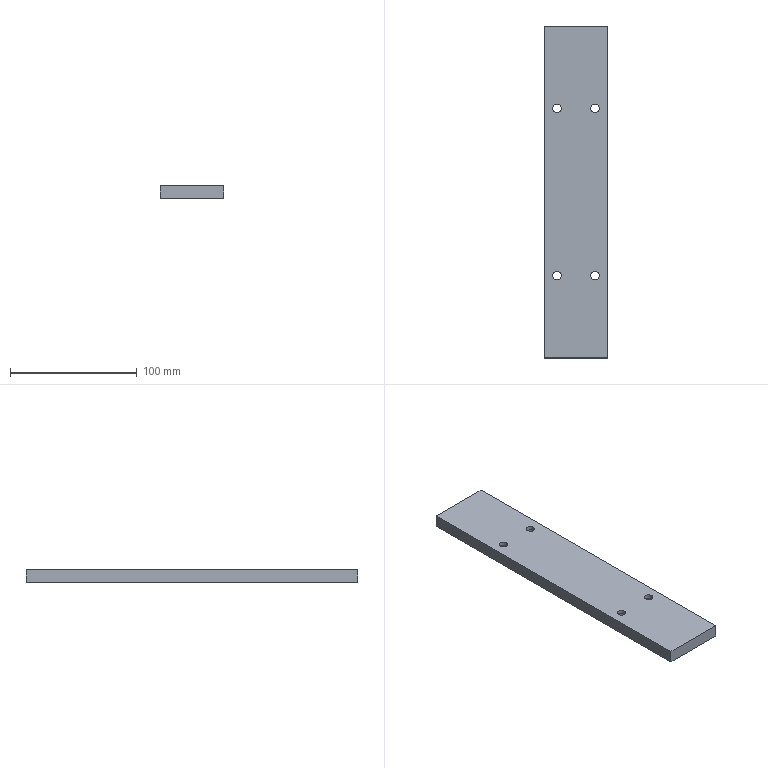Part | SolidWorks | features BaseBody 1 | 1 solid | 26 faces | box 50 x 262 x 10 mm | volume 127977 mm3 | cylinder 16 | plane 10 | commonest cylinder face diameters 6.6 x8 11 x8
STEP:
#1=CARTESIAN_POINT('',(-9.5,309.,-233.2));
#2=VERTEX_POINT('',#1);
#3=CARTESIAN_POINT('',(-20.5,309.,-233.2));
#4=VERTEX_POINT('',#3);
#5=CARTESIAN_POINT('',(-15.,309.,-233.2));
#6=DIRECTION('',(0.,0.,-1.));
#7=DIRECTION('',(-1.,0.,0.));
#8=AXIS2_PLACEMENT_3D('',#5,#6,#7);
#9=CIRCLE('',#8,5.5);
#10=EDGE_CURVE('',#2,#4,#9,.T.);
#11=ORIENTED_EDGE('',*,*,#10,.F.);
#12=CARTESIAN_POINT('',(-9.5,309.,-240.));
#13=VERTEX_POINT('',#12);
#14=CARTESIAN_POINT('',(-9.5,309.,-240.));
#15=DIRECTION('',(0.,0.,-1.));
#16=VECTOR('',#15,1000.);
#17=LINE('',#14,#16);
#18=EDGE_CURVE('',#2,#13,#17,.T.);
#19=ORIENTED_EDGE('',*,*,#18,.T.);
#20=CARTESIAN_POINT('',(-20.5,309.,-240.));
#21=VERTEX_POINT('',#20);
#22=CARTESIAN_POINT('',(-15.,309.,-240.));
#23=DIRECTION('',(0.,0.,-1.));
#24=DIRECTION('',(-1.,0.,0.));
#25=AXIS2_PLACEMENT_3D('',#22,#23,#24);
#26=CIRCLE('',#25,5.5);
#27=EDGE_CURVE('',#13,#21,#26,.T.);
#28=ORIENTED_EDGE('',*,*,#27,.T.);
#29=CARTESIAN_POINT('',(-20.5,309.,-240.));
#30=DIRECTION('',(0.,0.,-1.));
#31=VECTOR('',#30,1000.);
#32=LINE('',#29,#31);
#33=EDGE_CURVE('',#4,#21,#32,.T.);
#34=ORIENTED_EDGE('',*,*,#33,.F.);
#35=EDGE_LOOP('',(#11,#19,#28,#34));
#36=FACE_OUTER_BOUND('',#35,.T.);
#37=CARTESIAN_POINT('',(-15.,309.,-240.));
#38=DIRECTION('',(0.,0.,-1.));
#39=DIRECTION('',(-1.,0.,0.));
#40=AXIS2_PLACEMENT_3D('',#37,#38,#39);
#41=CYLINDRICAL_SURFACE('',#40,5.5);
#42=ADVANCED_FACE('',(#36),#41,.F.);
#43=CARTESIAN_POINT('',(-11.7,309.,-230.));
#44=VERTEX_POINT('',#43);
#45=CARTESIAN_POINT('',(-18.3,309.,-230.));
#46=VERTEX_POINT('',#45);
#47=CARTESIAN_POINT('',(-15.,309.,-230.));
#48=DIRECTION('',(0.,0.,-1.));
#49=DIRECTION('',(-1.,0.,0.));
#50=AXIS2_PLACEMENT_3D('',#47,#48,#49);
#51=CIRCLE('',#50,3.3);
#52=EDGE_CURVE('',#44,#46,#51,.T.);
#53=ORIENTED_EDGE('',*,*,#52,.F.);
#54=CARTESIAN_POINT('',(-11.7,309.,-233.2));
#55=VERTEX_POINT('',#54);
#56=CARTESIAN_POINT('',(-11.7,309.,-240.));
#57=DIRECTION('',(0.,0.,-1.));
#58=VECTOR('',#57,1000.);
#59=LINE('',#56,#58);
#60=EDGE_CURVE('',#44,#55,#59,.T.);
#61=ORIENTED_EDGE('',*,*,#60,.T.);
#62=CARTESIAN_POINT('',(-18.3,309.,-233.2));
#63=VERTEX_POINT('',#62);
#64=CARTESIAN_POINT('',(-15.,309.,-233.2));
#65=DIRECTION('',(0.,0.,-1.));
#66=DIRECTION('',(-1.,0.,0.));
#67=AXIS2_PLACEMENT_3D('',#64,#65,#66);
#68=CIRCLE('',#67,3.3);
#69=EDGE_CURVE('',#55,#63,#68,.T.);
#70=ORIENTED_EDGE('',*,*,#69,.T.);
#71=CARTESIAN_POINT('',(-18.3,309.,-240.));
#72=DIRECTION('',(0.,0.,-1.));
#73=VECTOR('',#72,1000.);
#74=LINE('',#71,#73);
#75=EDGE_CURVE('',#46,#63,#74,.T.);
#76=ORIENTED_EDGE('',*,*,#75,.F.);
#77=EDGE_LOOP('',(#53,#61,#70,#76));
#78=FACE_OUTER_BOUND('',#77,.T.);
#79=CARTESIAN_POINT('',(-15.,309.,-240.));
#80=DIRECTION('',(0.,0.,-1.));
#81=DIRECTION('',(-1.,0.,0.));
#82=AXIS2_PLACEMENT_3D('',#79,#80,#81);
#83=CYLINDRICAL_SURFACE('',#82,3.3);
#84=ADVANCED_FACE('',(#78),#83,.F.);
#85=CARTESIAN_POINT('',(20.5,309.,-233.2));
#86=VERTEX_POINT('',#85);
#87=CARTESIAN_POINT('',(9.5,309.,-233.2));
#88=VERTEX_POINT('',#87);
#89=CARTESIAN_POINT('',(15.,309.,-233.2));
#90=DIRECTION('',(0.,0.,-1.));
#91=DIRECTION('',(-1.,0.,0.));
#92=AXIS2_PLACEMENT_3D('',#89,#90,#91);
#93=CIRCLE('',#92,5.5);
#94=EDGE_CURVE('',#86,#88,#93,.T.);
#95=ORIENTED_EDGE('',*,*,#94,.F.);
#96=CARTESIAN_POINT('',(20.5,309.,-240.));
#97=VERTEX_POINT('',#96);
#98=CARTESIAN_POINT('',(20.5,309.,-240.));
#99=DIRECTION('',(0.,0.,-1.));
#100=VECTOR('',#99,1000.);
#101=LINE('',#98,#100);
#102=EDGE_CURVE('',#86,#97,#101,.T.);
#103=ORIENTED_EDGE('',*,*,#102,.T.);
#104=CARTESIAN_POINT('',(9.5,309.,-240.));
#105=VERTEX_POINT('',#104);
#106=CARTESIAN_POINT('',(15.,309.,-240.));
#107=DIRECTION('',(0.,0.,-1.));
#108=DIRECTION('',(-1.,0.,0.));
#109=AXIS2_PLACEMENT_3D('',#106,#107,#108);
#110=CIRCLE('',#109,5.5);
#111=EDGE_CURVE('',#97,#105,#110,.T.);
#112=ORIENTED_EDGE('',*,*,#111,.T.);
#113=CARTESIAN_POINT('',(9.5,309.,-240.));
#114=DIRECTION('',(0.,0.,-1.));
#115=VECTOR('',#114,1000.);
#116=LINE('',#113,#115);
#117=EDGE_CURVE('',#88,#105,#116,.T.);
#118=ORIENTED_EDGE('',*,*,#117,.F.);
#119=EDGE_LOOP('',(#95,#103,#112,#118));
#120=FACE_OUTER_BOUND('',#119,.T.);
#121=CARTESIAN_POINT('',(15.,309.,-240.));
#122=DIRECTION('',(0.,0.,-1.));
#123=DIRECTION('',(-1.,0.,0.));
#124=AXIS2_PLACEMENT_3D('',#121,#122,#123);
#125=CYLINDRICAL_SURFACE('',#124,5.5);
#126=ADVANCED_FACE('',(#120),#125,.F.);
#127=CARTESIAN_POINT('',(18.3,309.,-230.));
#128=VERTEX_POINT('',#127);
#129=CARTESIAN_POINT('',(11.7,309.,-230.));
#130=VERTEX_POINT('',#129);
#131=CARTESIAN_POINT('',(15.,309.,-230.));
#132=DIRECTION('',(0.,0.,-1.));
#133=DIRECTION('',(-1.,0.,0.));
#134=AXIS2_PLACEMENT_3D('',#131,#132,#133);
#135=CIRCLE('',#134,3.3);
#136=EDGE_CURVE('',#128,#130,#135,.T.);
#137=ORIENTED_EDGE('',*,*,#136,.F.);
#138=CARTESIAN_POINT('',(18.3,309.,-233.2));
#139=VERTEX_POINT('',#138);
#140=CARTESIAN_POINT('',(18.3,309.,-240.));
#141=DIRECTION('',(0.,0.,-1.));
#142=VECTOR('',#141,1000.);
#143=LINE('',#140,#142);
#144=EDGE_CURVE('',#128,#139,#143,.T.);
#145=ORIENTED_EDGE('',*,*,#144,.T.);
#146=CARTESIAN_POINT('',(11.7,309.,-233.2));
#147=VERTEX_POINT('',#146);
#148=CARTESIAN_POINT('',(15.,309.,-233.2));
#149=DIRECTION('',(0.,0.,-1.));
#150=DIRECTION('',(-1.,0.,0.));
#151=AXIS2_PLACEMENT_3D('',#148,#149,#150);
#152=CIRCLE('',#151,3.3);
#153=EDGE_CURVE('',#139,#147,#152,.T.);
#154=ORIENTED_EDGE('',*,*,#153,.T.);
#155=CARTESIAN_POINT('',(11.7,309.,-240.));
#156=DIRECTION('',(0.,0.,-1.));
#157=VECTOR('',#156,1000.);
#158=LINE('',#155,#157);
#159=EDGE_CURVE('',#130,#147,#158,.T.);
#160=ORIENTED_EDGE('',*,*,#159,.F.);
#161=EDGE_LOOP('',(#137,#145,#154,#160));
#162=FACE_OUTER_BOUND('',#161,.T.);
#163=CARTESIAN_POINT('',(15.,309.,-240.));
#164=DIRECTION('',(0.,0.,-1.));
#165=DIRECTION('',(-1.,0.,0.));
#166=AXIS2_PLACEMENT_3D('',#163,#164,#165);
#167=CYLINDRICAL_SURFACE('',#166,3.3);
#168=ADVANCED_FACE('',(#162),#167,.F.);
#169=CARTESIAN_POINT('',(18.3,441.,-230.));
#170=VERTEX_POINT('',#169);
#171=CARTESIAN_POINT('',(11.7,441.,-230.));
#172=VERTEX_POINT('',#171);
#173=CARTESIAN_POINT('',(15.,441.,-230.));
#174=DIRECTION('',(0.,0.,-1.));
#175=DIRECTION('',(-1.,0.,0.));
#176=AXIS2_PLACEMENT_3D('',#173,#174,#175);
#177=CIRCLE('',#176,3.3);
#178=EDGE_CURVE('',#170,#172,#177,.T.);
#179=ORIENTED_EDGE('',*,*,#178,.F.);
#180=CARTESIAN_POINT('',(18.3,441.,-233.2));
#181=VERTEX_POINT('',#180);
#182=CARTESIAN_POINT('',(18.3,441.,-240.));
#183=DIRECTION('',(0.,0.,-1.));
#184=VECTOR('',#183,1000.);
#185=LINE('',#182,#184);
#186=EDGE_CURVE('',#170,#181,#185,.T.);
#187=ORIENTED_EDGE('',*,*,#186,.T.);
#188=CARTESIAN_POINT('',(11.7,441.,-233.2));
#189=VERTEX_POINT('',#188);
#190=CARTESIAN_POINT('',(15.,441.,-233.2));
#191=DIRECTION('',(0.,0.,-1.));
#192=DIRECTION('',(-1.,0.,0.));
#193=AXIS2_PLACEMENT_3D('',#190,#191,#192);
#194=CIRCLE('',#193,3.3);
#195=EDGE_CURVE('',#181,#189,#194,.T.);
#196=ORIENTED_EDGE('',*,*,#195,.T.);
#197=CARTESIAN_POINT('',(11.7,441.,-240.));
#198=DIRECTION('',(0.,0.,-1.));
#199=VECTOR('',#198,1000.);
#200=LINE('',#197,#199);
#201=EDGE_CURVE('',#172,#189,#200,.T.);
#202=ORIENTED_EDGE('',*,*,#201,.F.);
#203=EDGE_LOOP('',(#179,#187,#196,#202));
#204=FACE_OUTER_BOUND('',#203,.T.);
#205=CARTESIAN_POINT('',(15.,441.,-240.));
#206=DIRECTION('',(0.,0.,-1.));
#207=DIRECTION('',(-1.,0.,0.));
#208=AXIS2_PLACEMENT_3D('',#205,#206,#207);
#209=CYLINDRICAL_SURFACE('',#208,3.3);
#210=ADVANCED_FACE('',(#204),#209,.F.);
#211=CARTESIAN_POINT('',(20.5,441.,-233.2));
#212=VERTEX_POINT('',#211);
#213=CARTESIAN_POINT('',(9.5,441.,-233.2));
#214=VERTEX_POINT('',#213);
#215=CARTESIAN_POINT('',(15.,441.,-233.2));
#216=DIRECTION('',(0.,0.,-1.));
#217=DIRECTION('',(-1.,0.,0.));
#218=AXIS2_PLACEMENT_3D('',#215,#216,#217);
#219=CIRCLE('',#218,5.5);
#220=EDGE_CURVE('',#212,#214,#219,.T.);
#221=ORIENTED_EDGE('',*,*,#220,.F.);
#222=CARTESIAN_POINT('',(20.5,441.,-240.));
#223=VERTEX_POINT('',#222);
#224=CARTESIAN_POINT('',(20.5,441.,-240.));
#225=DIRECTION('',(0.,0.,-1.));
#226=VECTOR('',#225,1000.);
#227=LINE('',#224,#226);
#228=EDGE_CURVE('',#212,#223,#227,.T.);
#229=ORIENTED_EDGE('',*,*,#228,.T.);
#230=CARTESIAN_POINT('',(9.5,441.,-240.));
#231=VERTEX_POINT('',#230);
#232=CARTESIAN_POINT('',(15.,441.,-240.));
#233=DIRECTION('',(0.,0.,-1.));
#234=DIRECTION('',(-1.,0.,0.));
#235=AXIS2_PLACEMENT_3D('',#232,#233,#234);
#236=CIRCLE('',#235,5.5);
#237=EDGE_CURVE('',#223,#231,#236,.T.);
#238=ORIENTED_EDGE('',*,*,#237,.T.);
#239=CARTESIAN_POINT('',(9.5,441.,-240.));
#240=DIRECTION('',(0.,0.,-1.));
#241=VECTOR('',#240,1000.);
#242=LINE('',#239,#241);
#243=EDGE_CURVE('',#214,#231,#242,.T.);
#244=ORIENTED_EDGE('',*,*,#243,.F.);
#245=EDGE_LOOP('',(#221,#229,#238,#244));
#246=FACE_OUTER_BOUND('',#245,.T.);
#247=CARTESIAN_POINT('',(15.,441.,-240.));
#248=DIRECTION('',(0.,0.,-1.));
#249=DIRECTION('',(-1.,0.,0.));
#250=AXIS2_PLACEMENT_3D('',#247,#248,#249);
#251=CYLINDRICAL_SURFACE('',#250,5.5);
#252=ADVANCED_FACE('',(#246),#251,.F.);
#253=CARTESIAN_POINT('',(-11.7,441.,-230.));
#254=VERTEX_POINT('',#253);
#255=CARTESIAN_POINT('',(-18.3,441.,-230.));
#256=VERTEX_POINT('',#255);
#257=CARTESIAN_POINT('',(-15.,441.,-230.));
#258=DIRECTION('',(0.,0.,-1.));
#259=DIRECTION('',(-1.,0.,0.));
#260=AXIS2_PLACEMENT_3D('',#257,#258,#259);
#261=CIRCLE('',#260,3.3);
#262=EDGE_CURVE('',#254,#256,#261,.T.);
#263=ORIENTED_EDGE('',*,*,#262,.F.);
#264=CARTESIAN_POINT('',(-11.7,441.,-233.2));
#265=VERTEX_POINT('',#264);
#266=CARTESIAN_POINT('',(-11.7,441.,-240.));
#267=DIRECTION('',(0.,0.,-1.));
#268=VECTOR('',#267,1000.);
#269=LINE('',#266,#268);
#270=EDGE_CURVE('',#254,#265,#269,.T.);
#271=ORIENTED_EDGE('',*,*,#270,.T.);
#272=CARTESIAN_POINT('',(-18.3,441.,-233.2));
#273=VERTEX_POINT('',#272);
#274=CARTESIAN_POINT('',(-15.,441.,-233.2));
#275=DIRECTION('',(0.,0.,-1.));
#276=DIRECTION('',(-1.,0.,0.));
#277=AXIS2_PLACEMENT_3D('',#274,#275,#276);
#278=CIRCLE('',#277,3.3);
#279=EDGE_CURVE('',#265,#273,#278,.T.);
#280=ORIENTED_EDGE('',*,*,#279,.T.);
#281=CARTESIAN_POINT('',(-18.3,441.,-240.));
#282=DIRECTION('',(0.,0.,-1.));
#283=VECTOR('',#282,1000.);
#284=LINE('',#281,#283);
#285=EDGE_CURVE('',#256,#273,#284,.T.);
#286=ORIENTED_EDGE('',*,*,#285,.F.);
#287=EDGE_LOOP('',(#263,#271,#280,#286));
#288=FACE_OUTER_BOUND('',#287,.T.);
#289=CARTESIAN_POINT('',(-15.,441.,-240.));
#290=DIRECTION('',(0.,0.,-1.));
#291=DIRECTION('',(-1.,0.,0.));
#292=AXIS2_PLACEMENT_3D('',#289,#290,#291);
#293=CYLINDRICAL_SURFACE('',#292,3.3);
#294=ADVANCED_FACE('',(#288),#293,.F.);
#295=CARTESIAN_POINT('',(-9.5,441.,-233.2));
#296=VERTEX_POINT('',#295);
#297=CARTESIAN_POINT('',(-20.5,441.,-233.2));
#298=VERTEX_POINT('',#297);
#299=CARTESIAN_POINT('',(-15.,441.,-233.2));
#300=DIRECTION('',(0.,0.,-1.));
#301=DIRECTION('',(-1.,0.,0.));
#302=AXIS2_PLACEMENT_3D('',#299,#300,#301);
#303=CIRCLE('',#302,5.5);
#304=EDGE_CURVE('',#296,#298,#303,.T.);
#305=ORIENTED_EDGE('',*,*,#304,.F.);
#306=CARTESIAN_POINT('',(-9.5,441.,-240.));
#307=VERTEX_POINT('',#306);
#308=CARTESIAN_POINT('',(-9.5,441.,-240.));
#309=DIRECTION('',(0.,0.,-1.));
#310=VECTOR('',#309,1000.);
#311=LINE('',#308,#310);
#312=EDGE_CURVE('',#296,#307,#311,.T.);
#313=ORIENTED_EDGE('',*,*,#312,.T.);
#314=CARTESIAN_POINT('',(-20.5,441.,-240.));
#315=VERTEX_POINT('',#314);
#316=CARTESIAN_POINT('',(-15.,441.,-240.));
#317=DIRECTION('',(0.,0.,-1.));
#318=DIRECTION('',(-1.,0.,0.));
#319=AXIS2_PLACEMENT_3D('',#316,#317,#318);
#320=CIRCLE('',#319,5.5);
#321=EDGE_CURVE('',#307,#315,#320,.T.);
#322=ORIENTED_EDGE('',*,*,#321,.T.);
#323=CARTESIAN_POINT('',(-20.5,441.,-240.));
#324=DIRECTION('',(0.,0.,-1.));
#325=VECTOR('',#324,1000.);
#326=LINE('',#323,#325);
#327=EDGE_CURVE('',#298,#315,#326,.T.);
#328=ORIENTED_EDGE('',*,*,#327,.F.);
#329=EDGE_LOOP('',(#305,#313,#322,#328));
#330=FACE_OUTER_BOUND('',#329,.T.);
#331=CARTESIAN_POINT('',(-15.,441.,-240.));
#332=DIRECTION('',(0.,0.,-1.));
#333=DIRECTION('',(-1.,0.,0.));
#334=AXIS2_PLACEMENT_3D('',#331,#332,#333);
#335=CYLINDRICAL_SURFACE('',#334,5.5);
#336=ADVANCED_FACE('',(#330),#335,.F.);
#337=CARTESIAN_POINT('',(-25.,244.,-240.));
#338=VERTEX_POINT('',#337);
#339=CARTESIAN_POINT('',(25.,244.,-240.));
#340=VERTEX_POINT('',#339);
#341=CARTESIAN_POINT('',(25.,244.,-240.));
#342=DIRECTION('',(1.,0.,0.));
#343=VECTOR('',#342,1000.);
#344=LINE('',#341,#343);
#345=EDGE_CURVE('',#338,#340,#344,.T.);
#346=ORIENTED_EDGE('',*,*,#345,.T.);
#347=CARTESIAN_POINT('',(25.,244.,-230.));
#348=VERTEX_POINT('',#347);
#349=CARTESIAN_POINT('',(25.,244.,-230.));
#350=DIRECTION('',(0.,0.,1.));
#351=VECTOR('',#350,1000.);
#352=LINE('',#349,#351);
#353=EDGE_CURVE('',#340,#348,#352,.T.);
#354=ORIENTED_EDGE('',*,*,#353,.T.);
#355=CARTESIAN_POINT('',(-25.,244.,-230.));
#356=VERTEX_POINT('',#355);
#357=CARTESIAN_POINT('',(25.,244.,-230.));
#358=DIRECTION('',(1.,0.,0.));
#359=VECTOR('',#358,1000.);
#360=LINE('',#357,#359);
#361=EDGE_CURVE('',#356,#348,#360,.T.);
#362=ORIENTED_EDGE('',*,*,#361,.F.);
#363=CARTESIAN_POINT('',(-25.,244.,-230.));
#364=DIRECTION('',(0.,0.,1.));
#365=VECTOR('',#364,1000.);
#366=LINE('',#363,#365);
#367=EDGE_CURVE('',#338,#356,#366,.T.);
#368=ORIENTED_EDGE('',*,*,#367,.F.);
#369=EDGE_LOOP('',(#346,#354,#362,#368));
#370=FACE_OUTER_BOUND('',#369,.T.);
#371=CARTESIAN_POINT('',(11453.619,244.,-234.));
#372=DIRECTION('',(0.,1.,0.));
#373=DIRECTION('',(1.,0.,0.));
#374=AXIS2_PLACEMENT_3D('',#371,#372,#373);
#375=PLANE('',#374);
#376=ADVANCED_FACE('',(#370),#375,.F.);
#377=CARTESIAN_POINT('',(25.,506.,-240.));
#378=VERTEX_POINT('',#377);
#379=CARTESIAN_POINT('',(-25.,506.,-240.));
#380=VERTEX_POINT('',#379);
#381=CARTESIAN_POINT('',(25.,506.,-240.));
#382=DIRECTION('',(-1.,0.,0.));
#383=VECTOR('',#382,1000.);
#384=LINE('',#381,#383);
#385=EDGE_CURVE('',#378,#380,#384,.T.);
#386=ORIENTED_EDGE('',*,*,#385,.T.);
#387=CARTESIAN_POINT('',(-25.,506.,-230.));
#388=VERTEX_POINT('',#387);
#389=CARTESIAN_POINT('',(-25.,506.,-230.));
#390=DIRECTION('',(0.,0.,1.));
#391=VECTOR('',#390,1000.);
#392=LINE('',#389,#391);
#393=EDGE_CURVE('',#380,#388,#392,.T.);
#394=ORIENTED_EDGE('',*,*,#393,.T.);
#395=CARTESIAN_POINT('',(25.,506.,-230.));
#396=VERTEX_POINT('',#395);
#397=CARTESIAN_POINT('',(25.,506.,-230.));
#398=DIRECTION('',(-1.,0.,0.));
#399=VECTOR('',#398,1000.);
#400=LINE('',#397,#399);
#401=EDGE_CURVE('',#396,#388,#400,.T.);
#402=ORIENTED_EDGE('',*,*,#401,.F.);
#403=CARTESIAN_POINT('',(25.,506.,-230.));
#404=DIRECTION('',(0.,0.,1.));
#405=VECTOR('',#404,1000.);
#406=LINE('',#403,#405);
#407=EDGE_CURVE('',#378,#396,#406,.T.);
#408=ORIENTED_EDGE('',*,*,#407,.F.);
#409=EDGE_LOOP('',(#386,#394,#402,#408));
#410=FACE_OUTER_BOUND('',#409,.T.);
#411=CARTESIAN_POINT('',(-9973.619,506.,-234.));
#412=DIRECTION('',(0.,-1.,0.));
#413=DIRECTION('',(0.,0.,-1.));
#414=AXIS2_PLACEMENT_3D('',#411,#412,#413);
#415=PLANE('',#414);
#416=ADVANCED_FACE('',(#410),#415,.F.);
#417=CARTESIAN_POINT('',(-15.,309.,-233.2));
#418=DIRECTION('',(0.,0.,-1.));
#419=DIRECTION('',(-1.,0.,0.));
#420=AXIS2_PLACEMENT_3D('',#417,#418,#419);
#421=CIRCLE('',#420,3.3);
#422=EDGE_CURVE('',#63,#55,#421,.T.);
#423=ORIENTED_EDGE('',*,*,#422,.F.);
#424=ORIENTED_EDGE('',*,*,#69,.F.);
#425=EDGE_LOOP('',(#423,#424));
#426=FACE_BOUND('',#425,.T.);
#427=CARTESIAN_POINT('',(-15.,309.,-233.2));
#428=DIRECTION('',(0.,0.,-1.));
#429=DIRECTION('',(-1.,0.,0.));
#430=AXIS2_PLACEMENT_3D('',#427,#428,#429);
#431=CIRCLE('',#430,5.5);
#432=EDGE_CURVE('',#4,#2,#431,.T.);
#433=ORIENTED_EDGE('',*,*,#432,.T.);
#434=ORIENTED_EDGE('',*,*,#10,.T.);
#435=EDGE_LOOP('',(#433,#434));
#436=FACE_OUTER_BOUND('',#435,.T.);
#437=CARTESIAN_POINT('',(-11.7,309.,-233.2));
#438=DIRECTION('',(0.,0.,1.));
#439=DIRECTION('',(1.,0.,0.));
#440=AXIS2_PLACEMENT_3D('',#437,#438,#439);
#441=PLANE('',#440);
#442=ADVANCED_FACE('',(#426,#436),#441,.F.);
#443=CARTESIAN_POINT('',(15.,309.,-233.2));
#444=DIRECTION('',(0.,0.,-1.));
#445=DIRECTION('',(-1.,0.,0.));
#446=AXIS2_PLACEMENT_3D('',#443,#444,#445);
#447=CIRCLE('',#446,3.3);
#448=EDGE_CURVE('',#147,#139,#447,.T.);
#449=ORIENTED_EDGE('',*,*,#448,.F.);
#450=ORIENTED_EDGE('',*,*,#153,.F.);
#451=EDGE_LOOP('',(#449,#450));
#452=FACE_BOUND('',#451,.T.);
#453=CARTESIAN_POINT('',(15.,309.,-233.2));
#454=DIRECTION('',(0.,0.,-1.));
#455=DIRECTION('',(-1.,0.,0.));
#456=AXIS2_PLACEMENT_3D('',#453,#454,#455);
#457=CIRCLE('',#456,5.5);
#458=EDGE_CURVE('',#88,#86,#457,.T.);
#459=ORIENTED_EDGE('',*,*,#458,.T.);
#460=ORIENTED_EDGE('',*,*,#94,.T.);
#461=EDGE_LOOP('',(#459,#460));
#462=FACE_OUTER_BOUND('',#461,.T.);
#463=CARTESIAN_POINT('',(18.3,309.,-233.2));
#464=DIRECTION('',(0.,0.,1.));
#465=DIRECTION('',(1.,0.,0.));
#466=AXIS2_PLACEMENT_3D('',#463,#464,#465);
#467=PLANE('',#466);
#468=ADVANCED_FACE('',(#452,#462),#467,.F.);
#469=CARTESIAN_POINT('',(-15.,441.,-240.));
#470=DIRECTION('',(0.,0.,-1.));
#471=DIRECTION('',(-1.,0.,0.));
#472=AXIS2_PLACEMENT_3D('',#469,#470,#471);
#473=CIRCLE('',#472,5.5);
#474=EDGE_CURVE('',#315,#307,#473,.T.);
#475=ORIENTED_EDGE('',*,*,#474,.F.);
#476=ORIENTED_EDGE('',*,*,#321,.F.);
#477=EDGE_LOOP('',(#475,#476));
#478=FACE_BOUND('',#477,.T.);
#479=CARTESIAN_POINT('',(15.,441.,-240.));
#480=DIRECTION('',(0.,0.,-1.));
#481=DIRECTION('',(-1.,0.,0.));
#482=AXIS2_PLACEMENT_3D('',#479,#480,#481);
#483=CIRCLE('',#482,5.5);
#484=EDGE_CURVE('',#231,#223,#483,.T.);
#485=ORIENTED_EDGE('',*,*,#484,.F.);
#486=ORIENTED_EDGE('',*,*,#237,.F.);
#487=EDGE_LOOP('',(#485,#486));
#488=FACE_BOUND('',#487,.T.);
#489=CARTESIAN_POINT('',(15.,309.,-240.));
#490=DIRECTION('',(0.,0.,-1.));
#491=DIRECTION('',(-1.,0.,0.));
#492=AXIS2_PLACEMENT_3D('',#489,#490,#491);
#493=CIRCLE('',#492,5.5);
#494=EDGE_CURVE('',#105,#97,#493,.T.);
#495=ORIENTED_EDGE('',*,*,#494,.F.);
#496=ORIENTED_EDGE('',*,*,#111,.F.);
#497=EDGE_LOOP('',(#495,#496));
#498=FACE_BOUND('',#497,.T.);
#499=CARTESIAN_POINT('',(-15.,309.,-240.));
#500=DIRECTION('',(0.,0.,-1.));
#501=DIRECTION('',(-1.,0.,0.));
#502=AXIS2_PLACEMENT_3D('',#499,#500,#501);
#503=CIRCLE('',#502,5.5);
#504=EDGE_CURVE('',#21,#13,#503,.T.);
#505=ORIENTED_EDGE('',*,*,#504,.F.);
#506=ORIENTED_EDGE('',*,*,#27,.F.);
#507=EDGE_LOOP('',(#505,#506));
#508=FACE_BOUND('',#507,.T.);
#509=CARTESIAN_POINT('',(25.,496.,-240.));
#510=DIRECTION('',(0.,-1.,0.));
#511=VECTOR('',#510,1000.);
#512=LINE('',#509,#511);
#513=EDGE_CURVE('',#378,#340,#512,.T.);
#514=ORIENTED_EDGE('',*,*,#513,.T.);
#515=ORIENTED_EDGE('',*,*,#345,.F.);
#516=CARTESIAN_POINT('',(-25.,496.,-240.));
#517=DIRECTION('',(0.,1.,0.));
#518=VECTOR('',#517,1000.);
#519=LINE('',#516,#518);
#520=EDGE_CURVE('',#338,#380,#519,.T.);
#521=ORIENTED_EDGE('',*,*,#520,.T.);
#522=ORIENTED_EDGE('',*,*,#385,.F.);
#523=EDGE_LOOP('',(#514,#515,#521,#522));
#524=FACE_OUTER_BOUND('',#523,.T.);
#525=CARTESIAN_POINT('',(-1480.,0.,-240.));
#526=DIRECTION('',(0.,0.,-1.));
#527=DIRECTION('',(0.,-1.,0.));
#528=AXIS2_PLACEMENT_3D('',#525,#526,#527);
#529=PLANE('',#528);
#530=ADVANCED_FACE('',(#478,#488,#498,#508,#524),#529,.T.);
#531=CARTESIAN_POINT('',(-15.,441.,-230.));
#532=DIRECTION('',(0.,0.,-1.));
#533=DIRECTION('',(-1.,0.,0.));
#534=AXIS2_PLACEMENT_3D('',#531,#532,#533);
#535=CIRCLE('',#534,3.3);
#536=EDGE_CURVE('',#256,#254,#535,.T.);
#537=ORIENTED_EDGE('',*,*,#536,.T.);
#538=ORIENTED_EDGE('',*,*,#262,.T.);
#539=EDGE_LOOP('',(#537,#538));
#540=FACE_BOUND('',#539,.T.);
#541=CARTESIAN_POINT('',(15.,441.,-230.));
#542=DIRECTION('',(0.,0.,-1.));
#543=DIRECTION('',(-1.,0.,0.));
#544=AXIS2_PLACEMENT_3D('',#541,#542,#543);
#545=CIRCLE('',#544,3.3);
#546=EDGE_CURVE('',#172,#170,#545,.T.);
#547=ORIENTED_EDGE('',*,*,#546,.T.);
#548=ORIENTED_EDGE('',*,*,#178,.T.);
#549=EDGE_LOOP('',(#547,#548));
#550=FACE_BOUND('',#549,.T.);
#551=CARTESIAN_POINT('',(15.,309.,-230.));
#552=DIRECTION('',(0.,0.,-1.));
#553=DIRECTION('',(-1.,0.,0.));
#554=AXIS2_PLACEMENT_3D('',#551,#552,#553);
#555=CIRCLE('',#554,3.3);
#556=EDGE_CURVE('',#130,#128,#555,.T.);
#557=ORIENTED_EDGE('',*,*,#556,.T.);
#558=ORIENTED_EDGE('',*,*,#136,.T.);
#559=EDGE_LOOP('',(#557,#558));
#560=FACE_BOUND('',#559,.T.);
#561=CARTESIAN_POINT('',(-15.,309.,-230.));
#562=DIRECTION('',(0.,0.,-1.));
#563=DIRECTION('',(-1.,0.,0.));
#564=AXIS2_PLACEMENT_3D('',#561,#562,#563);
#565=CIRCLE('',#564,3.3);
#566=EDGE_CURVE('',#46,#44,#565,.T.);
#567=ORIENTED_EDGE('',*,*,#566,.T.);
#568=ORIENTED_EDGE('',*,*,#52,.T.);
#569=EDGE_LOOP('',(#567,#568));
#570=FACE_BOUND('',#569,.T.);
#571=CARTESIAN_POINT('',(25.,496.,-230.));
#572=DIRECTION('',(0.,-1.,0.));
#573=VECTOR('',#572,1000.);
#574=LINE('',#571,#573);
#575=EDGE_CURVE('',#396,#348,#574,.T.);
#576=ORIENTED_EDGE('',*,*,#575,.F.);
#577=ORIENTED_EDGE('',*,*,#401,.T.);
#578=CARTESIAN_POINT('',(-25.,496.,-230.));
#579=DIRECTION('',(0.,1.,0.));
#580=VECTOR('',#579,1000.);
#581=LINE('',#578,#580);
#582=EDGE_CURVE('',#356,#388,#581,.T.);
#583=ORIENTED_EDGE('',*,*,#582,.F.);
#584=ORIENTED_EDGE('',*,*,#361,.T.);
#585=EDGE_LOOP('',(#576,#577,#583,#584));
#586=FACE_OUTER_BOUND('',#585,.T.);
#587=CARTESIAN_POINT('',(-1480.,0.,-230.));
#588=DIRECTION('',(0.,0.,-1.));
#589=DIRECTION('',(0.,-1.,0.));
#590=AXIS2_PLACEMENT_3D('',#587,#588,#589);
#591=PLANE('',#590);
#592=ADVANCED_FACE('',(#540,#550,#560,#570,#586),#591,.F.);
#593=ORIENTED_EDGE('',*,*,#520,.F.);
#594=ORIENTED_EDGE('',*,*,#367,.T.);
#595=ORIENTED_EDGE('',*,*,#582,.T.);
#596=ORIENTED_EDGE('',*,*,#393,.F.);
#597=EDGE_LOOP('',(#593,#594,#595,#596));
#598=FACE_OUTER_BOUND('',#597,.T.);
#599=CARTESIAN_POINT('',(-25.,496.,-230.));
#600=DIRECTION('',(-1.,0.,0.));
#601=DIRECTION('',(0.,0.,1.));
#602=AXIS2_PLACEMENT_3D('',#599,#600,#601);
#603=PLANE('',#602);
#604=ADVANCED_FACE('',(#598),#603,.T.);
#605=ORIENTED_EDGE('',*,*,#513,.F.);
#606=ORIENTED_EDGE('',*,*,#407,.T.);
#607=ORIENTED_EDGE('',*,*,#575,.T.);
#608=ORIENTED_EDGE('',*,*,#353,.F.);
#609=EDGE_LOOP('',(#605,#606,#607,#608));
#610=FACE_OUTER_BOUND('',#609,.T.);
#611=CARTESIAN_POINT('',(25.,496.,-230.));
#612=DIRECTION('',(1.,0.,0.));
#613=DIRECTION('',(0.,1.,0.));
#614=AXIS2_PLACEMENT_3D('',#611,#612,#613);
#615=PLANE('',#614);
#616=ADVANCED_FACE('',(#610),#615,.T.);
#617=CARTESIAN_POINT('',(15.,441.,-233.2));
#618=DIRECTION('',(0.,0.,-1.));
#619=DIRECTION('',(-1.,0.,0.));
#620=AXIS2_PLACEMENT_3D('',#617,#618,#619);
#621=CIRCLE('',#620,3.3);
#622=EDGE_CURVE('',#189,#181,#621,.T.);
#623=ORIENTED_EDGE('',*,*,#622,.F.);
#624=ORIENTED_EDGE('',*,*,#195,.F.);
#625=EDGE_LOOP('',(#623,#624));
#626=FACE_BOUND('',#625,.T.);
#627=CARTESIAN_POINT('',(15.,441.,-233.2));
#628=DIRECTION('',(0.,0.,-1.));
#629=DIRECTION('',(-1.,0.,0.));
#630=AXIS2_PLACEMENT_3D('',#627,#628,#629);
#631=CIRCLE('',#630,5.5);
#632=EDGE_CURVE('',#214,#212,#631,.T.);
#633=ORIENTED_EDGE('',*,*,#632,.T.);
#634=ORIENTED_EDGE('',*,*,#220,.T.);
#635=EDGE_LOOP('',(#633,#634));
#636=FACE_OUTER_BOUND('',#635,.T.);
#637=CARTESIAN_POINT('',(18.3,441.,-233.2));
#638=DIRECTION('',(0.,0.,1.));
#639=DIRECTION('',(1.,0.,0.));
#640=AXIS2_PLACEMENT_3D('',#637,#638,#639);
#641=PLANE('',#640);
#642=ADVANCED_FACE('',(#626,#636),#641,.F.);
#643=CARTESIAN_POINT('',(-15.,441.,-233.2));
#644=DIRECTION('',(0.,0.,-1.));
#645=DIRECTION('',(-1.,0.,0.));
#646=AXIS2_PLACEMENT_3D('',#643,#644,#645);
#647=CIRCLE('',#646,3.3);
#648=EDGE_CURVE('',#273,#265,#647,.T.);
#649=ORIENTED_EDGE('',*,*,#648,.F.);
#650=ORIENTED_EDGE('',*,*,#279,.F.);
#651=EDGE_LOOP('',(#649,#650));
#652=FACE_BOUND('',#651,.T.);
#653=CARTESIAN_POINT('',(-15.,441.,-233.2));
#654=DIRECTION('',(0.,0.,-1.));
#655=DIRECTION('',(-1.,0.,0.));
#656=AXIS2_PLACEMENT_3D('',#653,#654,#655);
#657=CIRCLE('',#656,5.5);
#658=EDGE_CURVE('',#298,#296,#657,.T.);
#659=ORIENTED_EDGE('',*,*,#658,.T.);
#660=ORIENTED_EDGE('',*,*,#304,.T.);
#661=EDGE_LOOP('',(#659,#660));
#662=FACE_OUTER_BOUND('',#661,.T.);
#663=CARTESIAN_POINT('',(-11.7,441.,-233.2));
#664=DIRECTION('',(0.,0.,1.));
#665=DIRECTION('',(1.,0.,0.));
#666=AXIS2_PLACEMENT_3D('',#663,#664,#665);
#667=PLANE('',#666);
#668=ADVANCED_FACE('',(#652,#662),#667,.F.);
#669=ORIENTED_EDGE('',*,*,#312,.F.);
#670=ORIENTED_EDGE('',*,*,#658,.F.);
#671=ORIENTED_EDGE('',*,*,#327,.T.);
#672=ORIENTED_EDGE('',*,*,#474,.T.);
#673=EDGE_LOOP('',(#669,#670,#671,#672));
#674=FACE_OUTER_BOUND('',#673,.T.);
#675=CARTESIAN_POINT('',(-15.,441.,-240.));
#676=DIRECTION('',(0.,0.,-1.));
#677=DIRECTION('',(-1.,0.,0.));
#678=AXIS2_PLACEMENT_3D('',#675,#676,#677);
#679=CYLINDRICAL_SURFACE('',#678,5.5);
#680=ADVANCED_FACE('',(#674),#679,.F.);
#681=ORIENTED_EDGE('',*,*,#270,.F.);
#682=ORIENTED_EDGE('',*,*,#536,.F.);
#683=ORIENTED_EDGE('',*,*,#285,.T.);
#684=ORIENTED_EDGE('',*,*,#648,.T.);
#685=EDGE_LOOP('',(#681,#682,#683,#684));
#686=FACE_OUTER_BOUND('',#685,.T.);
#687=CARTESIAN_POINT('',(-15.,441.,-240.));
#688=DIRECTION('',(0.,0.,-1.));
#689=DIRECTION('',(-1.,0.,0.));
#690=AXIS2_PLACEMENT_3D('',#687,#688,#689);
#691=CYLINDRICAL_SURFACE('',#690,3.3);
#692=ADVANCED_FACE('',(#686),#691,.F.);
#693=ORIENTED_EDGE('',*,*,#228,.F.);
#694=ORIENTED_EDGE('',*,*,#632,.F.);
#695=ORIENTED_EDGE('',*,*,#243,.T.);
#696=ORIENTED_EDGE('',*,*,#484,.T.);
#697=EDGE_LOOP('',(#693,#694,#695,#696));
#698=FACE_OUTER_BOUND('',#697,.T.);
#699=CARTESIAN_POINT('',(15.,441.,-240.));
#700=DIRECTION('',(0.,0.,-1.));
#701=DIRECTION('',(-1.,0.,0.));
#702=AXIS2_PLACEMENT_3D('',#699,#700,#701);
#703=CYLINDRICAL_SURFACE('',#702,5.5);
#704=ADVANCED_FACE('',(#698),#703,.F.);
#705=ORIENTED_EDGE('',*,*,#186,.F.);
#706=ORIENTED_EDGE('',*,*,#546,.F.);
#707=ORIENTED_EDGE('',*,*,#201,.T.);
#708=ORIENTED_EDGE('',*,*,#622,.T.);
#709=EDGE_LOOP('',(#705,#706,#707,#708));
#710=FACE_OUTER_BOUND('',#709,.T.);
#711=CARTESIAN_POINT('',(15.,441.,-240.));
#712=DIRECTION('',(0.,0.,-1.));
#713=DIRECTION('',(-1.,0.,0.));
#714=AXIS2_PLACEMENT_3D('',#711,#712,#713);
#715=CYLINDRICAL_SURFACE('',#714,3.3);
#716=ADVANCED_FACE('',(#710),#715,.F.);
#717=ORIENTED_EDGE('',*,*,#144,.F.);
#718=ORIENTED_EDGE('',*,*,#556,.F.);
#719=ORIENTED_EDGE('',*,*,#159,.T.);
#720=ORIENTED_EDGE('',*,*,#448,.T.);
#721=EDGE_LOOP('',(#717,#718,#719,#720));
#722=FACE_OUTER_BOUND('',#721,.T.);
#723=CARTESIAN_POINT('',(15.,309.,-240.));
#724=DIRECTION('',(0.,0.,-1.));
#725=DIRECTION('',(-1.,0.,0.));
#726=AXIS2_PLACEMENT_3D('',#723,#724,#725);
#727=CYLINDRICAL_SURFACE('',#726,3.3);
#728=ADVANCED_FACE('',(#722),#727,.F.);
#729=ORIENTED_EDGE('',*,*,#102,.F.);
#730=ORIENTED_EDGE('',*,*,#458,.F.);
#731=ORIENTED_EDGE('',*,*,#117,.T.);
#732=ORIENTED_EDGE('',*,*,#494,.T.);
#733=EDGE_LOOP('',(#729,#730,#731,#732));
#734=FACE_OUTER_BOUND('',#733,.T.);
#735=CARTESIAN_POINT('',(15.,309.,-240.));
#736=DIRECTION('',(0.,0.,-1.));
#737=DIRECTION('',(-1.,0.,0.));
#738=AXIS2_PLACEMENT_3D('',#735,#736,#737);
#739=CYLINDRICAL_SURFACE('',#738,5.5);
#740=ADVANCED_FACE('',(#734),#739,.F.);
#741=ORIENTED_EDGE('',*,*,#60,.F.);
#742=ORIENTED_EDGE('',*,*,#566,.F.);
#743=ORIENTED_EDGE('',*,*,#75,.T.);
#744=ORIENTED_EDGE('',*,*,#422,.T.);
#745=EDGE_LOOP('',(#741,#742,#743,#744));
#746=FACE_OUTER_BOUND('',#745,.T.);
#747=CARTESIAN_POINT('',(-15.,309.,-240.));
#748=DIRECTION('',(0.,0.,-1.));
#749=DIRECTION('',(-1.,0.,0.));
#750=AXIS2_PLACEMENT_3D('',#747,#748,#749);
#751=CYLINDRICAL_SURFACE('',#750,3.3);
#752=ADVANCED_FACE('',(#746),#751,.F.);
#753=ORIENTED_EDGE('',*,*,#18,.F.);
#754=ORIENTED_EDGE('',*,*,#432,.F.);
#755=ORIENTED_EDGE('',*,*,#33,.T.);
#756=ORIENTED_EDGE('',*,*,#504,.T.);
#757=EDGE_LOOP('',(#753,#754,#755,#756));
#758=FACE_OUTER_BOUND('',#757,.T.);
#759=CARTESIAN_POINT('',(-15.,309.,-240.));
#760=DIRECTION('',(0.,0.,-1.));
#761=DIRECTION('',(-1.,0.,0.));
#762=AXIS2_PLACEMENT_3D('',#759,#760,#761);
#763=CYLINDRICAL_SURFACE('',#762,5.5);
#764=ADVANCED_FACE('',(#758),#763,.F.);
#765=CLOSED_SHELL('',(#42,#84,#126,#168,#210,#252,#294,#336,#376,#416,#442,#468,#530,#592,#604,#616,#642,#668,#680,#692,#704,#716,#728,#740,#752,#764));
#766=MANIFOLD_SOLID_BREP('',#765);
#767=CARTESIAN_POINT('',(0.,0.,0.));
#768=DIRECTION('',(0.,0.,1.));
#769=DIRECTION('',(1.,0.,0.));
#770=AXIS2_PLACEMENT_3D('',#767,#768,#769);
#771=(LENGTH_UNIT()NAMED_UNIT(*)SI_UNIT(.MILLI.,.METRE.));
#772=UNCERTAINTY_MEASURE_WITH_UNIT(LENGTH_MEASURE(0.00001),#771,'','');
#773=(NAMED_UNIT(*)PLANE_ANGLE_UNIT()SI_UNIT($,.RADIAN.));
#774=(NAMED_UNIT(*)SI_UNIT($,.STERADIAN.)SOLID_ANGLE_UNIT());
#775=(GEOMETRIC_REPRESENTATION_CONTEXT(3)GLOBAL_UNCERTAINTY_ASSIGNED_CONTEXT((#772))GLOBAL_UNIT_ASSIGNED_CONTEXT((#771,#773,#774))REPRESENTATION_CONTEXT('',''));
#776=ADVANCED_BREP_SHAPE_REPRESENTATION('',(#766,#770),#775);